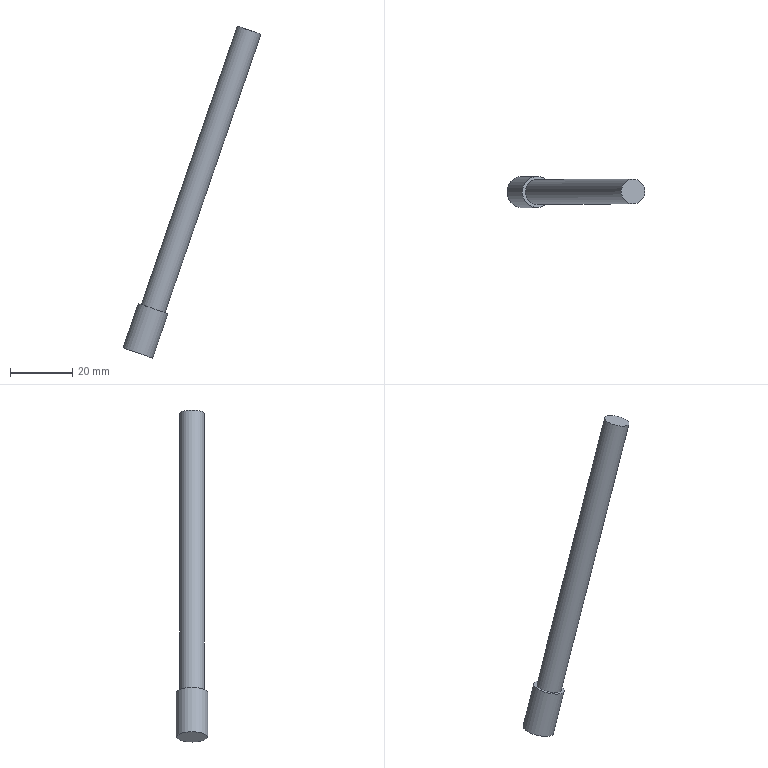Part | STEP file | solid 119 | 1 solid | 5 faces | box 44.094 x 10 x 106.274 mm | volume 5918 mm3 | plane 3 | cylinder 2 | commonest cylinder face diameters 8 x1 10 x1